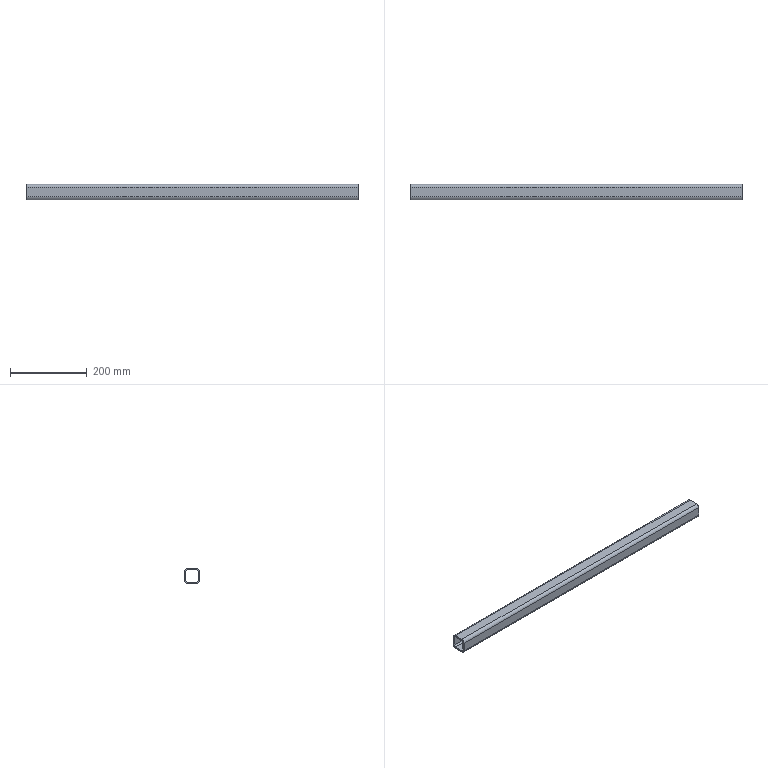Part | SolidWorks | features WeldMemberFeat 1, WeldmentFeature 1 | 1 solid | 18 faces | box 866 x 40 x 40 mm | volume 463134 mm3 | plane 10 | cylinder 8 | commonest cylinder face diameters 8 x4 16 x4
STEP:
#1=CARTESIAN_POINT('',(-433.,12.,-20.));
#2=VERTEX_POINT('',#1);
#3=CARTESIAN_POINT('',(-433.,20.,-12.));
#4=VERTEX_POINT('',#3);
#5=CARTESIAN_POINT('',(-433.,12.,-12.));
#6=DIRECTION('',(1.,0.,0.));
#7=DIRECTION('',(0.,0.,-1.));
#8=AXIS2_PLACEMENT_3D('',#5,#6,#7);
#9=CIRCLE('',#8,8.);
#10=EDGE_CURVE('',#2,#4,#9,.T.);
#11=ORIENTED_EDGE('',*,*,#10,.T.);
#12=CARTESIAN_POINT('',(433.,20.,-12.));
#13=VERTEX_POINT('',#12);
#14=CARTESIAN_POINT('',(433.,20.,-12.));
#15=DIRECTION('',(-1.,0.,0.));
#16=VECTOR('',#15,1000.);
#17=LINE('',#14,#16);
#18=EDGE_CURVE('',#13,#4,#17,.T.);
#19=ORIENTED_EDGE('',*,*,#18,.F.);
#20=CARTESIAN_POINT('',(433.,12.,-20.));
#21=VERTEX_POINT('',#20);
#22=CARTESIAN_POINT('',(433.,12.,-12.));
#23=DIRECTION('',(1.,0.,0.));
#24=DIRECTION('',(0.,0.,-1.));
#25=AXIS2_PLACEMENT_3D('',#22,#23,#24);
#26=CIRCLE('',#25,8.);
#27=EDGE_CURVE('',#21,#13,#26,.T.);
#28=ORIENTED_EDGE('',*,*,#27,.F.);
#29=CARTESIAN_POINT('',(433.,12.,-20.));
#30=DIRECTION('',(-1.,0.,0.));
#31=VECTOR('',#30,1000.);
#32=LINE('',#29,#31);
#33=EDGE_CURVE('',#21,#2,#32,.T.);
#34=ORIENTED_EDGE('',*,*,#33,.T.);
#35=EDGE_LOOP('',(#11,#19,#28,#34));
#36=FACE_OUTER_BOUND('',#35,.T.);
#37=CARTESIAN_POINT('',(433.,12.,-12.));
#38=DIRECTION('',(-1.,0.,0.));
#39=DIRECTION('',(0.,0.,1.));
#40=AXIS2_PLACEMENT_3D('',#37,#38,#39);
#41=CYLINDRICAL_SURFACE('',#40,8.);
#42=ADVANCED_FACE('',(#36),#41,.T.);
#43=CARTESIAN_POINT('',(-433.,20.,12.));
#44=VERTEX_POINT('',#43);
#45=CARTESIAN_POINT('',(-433.,20.,-12.));
#46=DIRECTION('',(0.,0.,1.));
#47=VECTOR('',#46,1000.);
#48=LINE('',#45,#47);
#49=EDGE_CURVE('',#4,#44,#48,.T.);
#50=ORIENTED_EDGE('',*,*,#49,.T.);
#51=CARTESIAN_POINT('',(433.,20.,12.));
#52=VERTEX_POINT('',#51);
#53=CARTESIAN_POINT('',(433.,20.,12.));
#54=DIRECTION('',(-1.,0.,0.));
#55=VECTOR('',#54,1000.);
#56=LINE('',#53,#55);
#57=EDGE_CURVE('',#52,#44,#56,.T.);
#58=ORIENTED_EDGE('',*,*,#57,.F.);
#59=CARTESIAN_POINT('',(433.,20.,-12.));
#60=DIRECTION('',(0.,0.,1.));
#61=VECTOR('',#60,1000.);
#62=LINE('',#59,#61);
#63=EDGE_CURVE('',#13,#52,#62,.T.);
#64=ORIENTED_EDGE('',*,*,#63,.F.);
#65=ORIENTED_EDGE('',*,*,#18,.T.);
#66=EDGE_LOOP('',(#50,#58,#64,#65));
#67=FACE_OUTER_BOUND('',#66,.T.);
#68=CARTESIAN_POINT('',(433.,20.,-12.));
#69=DIRECTION('',(0.,-1.,0.));
#70=DIRECTION('',(0.,0.,-1.));
#71=AXIS2_PLACEMENT_3D('',#68,#69,#70);
#72=PLANE('',#71);
#73=ADVANCED_FACE('',(#67),#72,.F.);
#74=CARTESIAN_POINT('',(-433.,12.,20.));
#75=VERTEX_POINT('',#74);
#76=CARTESIAN_POINT('',(-433.,12.,12.));
#77=DIRECTION('',(1.,0.,0.));
#78=DIRECTION('',(0.,0.,-1.));
#79=AXIS2_PLACEMENT_3D('',#76,#77,#78);
#80=CIRCLE('',#79,8.);
#81=EDGE_CURVE('',#44,#75,#80,.T.);
#82=ORIENTED_EDGE('',*,*,#81,.T.);
#83=CARTESIAN_POINT('',(433.,12.,20.));
#84=VERTEX_POINT('',#83);
#85=CARTESIAN_POINT('',(433.,12.,20.));
#86=DIRECTION('',(-1.,0.,0.));
#87=VECTOR('',#86,1000.);
#88=LINE('',#85,#87);
#89=EDGE_CURVE('',#84,#75,#88,.T.);
#90=ORIENTED_EDGE('',*,*,#89,.F.);
#91=CARTESIAN_POINT('',(433.,12.,12.));
#92=DIRECTION('',(1.,0.,0.));
#93=DIRECTION('',(0.,0.,-1.));
#94=AXIS2_PLACEMENT_3D('',#91,#92,#93);
#95=CIRCLE('',#94,8.);
#96=EDGE_CURVE('',#52,#84,#95,.T.);
#97=ORIENTED_EDGE('',*,*,#96,.F.);
#98=ORIENTED_EDGE('',*,*,#57,.T.);
#99=EDGE_LOOP('',(#82,#90,#97,#98));
#100=FACE_OUTER_BOUND('',#99,.T.);
#101=CARTESIAN_POINT('',(433.,12.,12.));
#102=DIRECTION('',(-1.,0.,0.));
#103=DIRECTION('',(0.,0.,1.));
#104=AXIS2_PLACEMENT_3D('',#101,#102,#103);
#105=CYLINDRICAL_SURFACE('',#104,8.);
#106=ADVANCED_FACE('',(#100),#105,.T.);
#107=CARTESIAN_POINT('',(-433.,-12.,20.));
#108=VERTEX_POINT('',#107);
#109=CARTESIAN_POINT('',(-433.,-12.,20.));
#110=DIRECTION('',(0.,-1.,0.));
#111=VECTOR('',#110,1000.);
#112=LINE('',#109,#111);
#113=EDGE_CURVE('',#75,#108,#112,.T.);
#114=ORIENTED_EDGE('',*,*,#113,.T.);
#115=CARTESIAN_POINT('',(433.,-12.,20.));
#116=VERTEX_POINT('',#115);
#117=CARTESIAN_POINT('',(433.,-12.,20.));
#118=DIRECTION('',(-1.,0.,0.));
#119=VECTOR('',#118,1000.);
#120=LINE('',#117,#119);
#121=EDGE_CURVE('',#116,#108,#120,.T.);
#122=ORIENTED_EDGE('',*,*,#121,.F.);
#123=CARTESIAN_POINT('',(433.,-12.,20.));
#124=DIRECTION('',(0.,-1.,0.));
#125=VECTOR('',#124,1000.);
#126=LINE('',#123,#125);
#127=EDGE_CURVE('',#84,#116,#126,.T.);
#128=ORIENTED_EDGE('',*,*,#127,.F.);
#129=ORIENTED_EDGE('',*,*,#89,.T.);
#130=EDGE_LOOP('',(#114,#122,#128,#129));
#131=FACE_OUTER_BOUND('',#130,.T.);
#132=CARTESIAN_POINT('',(433.,-12.,20.));
#133=DIRECTION('',(0.,0.,-1.));
#134=DIRECTION('',(-1.,0.,0.));
#135=AXIS2_PLACEMENT_3D('',#132,#133,#134);
#136=PLANE('',#135);
#137=ADVANCED_FACE('',(#131),#136,.F.);
#138=CARTESIAN_POINT('',(-433.,-20.,12.));
#139=VERTEX_POINT('',#138);
#140=CARTESIAN_POINT('',(-433.,-12.,12.));
#141=DIRECTION('',(1.,0.,0.));
#142=DIRECTION('',(0.,0.,-1.));
#143=AXIS2_PLACEMENT_3D('',#140,#141,#142);
#144=CIRCLE('',#143,8.);
#145=EDGE_CURVE('',#108,#139,#144,.T.);
#146=ORIENTED_EDGE('',*,*,#145,.T.);
#147=CARTESIAN_POINT('',(433.,-20.,12.));
#148=VERTEX_POINT('',#147);
#149=CARTESIAN_POINT('',(433.,-20.,12.));
#150=DIRECTION('',(-1.,0.,0.));
#151=VECTOR('',#150,1000.);
#152=LINE('',#149,#151);
#153=EDGE_CURVE('',#148,#139,#152,.T.);
#154=ORIENTED_EDGE('',*,*,#153,.F.);
#155=CARTESIAN_POINT('',(433.,-12.,12.));
#156=DIRECTION('',(1.,0.,0.));
#157=DIRECTION('',(0.,0.,-1.));
#158=AXIS2_PLACEMENT_3D('',#155,#156,#157);
#159=CIRCLE('',#158,8.);
#160=EDGE_CURVE('',#116,#148,#159,.T.);
#161=ORIENTED_EDGE('',*,*,#160,.F.);
#162=ORIENTED_EDGE('',*,*,#121,.T.);
#163=EDGE_LOOP('',(#146,#154,#161,#162));
#164=FACE_OUTER_BOUND('',#163,.T.);
#165=CARTESIAN_POINT('',(433.,-12.,12.));
#166=DIRECTION('',(-1.,0.,0.));
#167=DIRECTION('',(0.,0.,1.));
#168=AXIS2_PLACEMENT_3D('',#165,#166,#167);
#169=CYLINDRICAL_SURFACE('',#168,8.);
#170=ADVANCED_FACE('',(#164),#169,.T.);
#171=CARTESIAN_POINT('',(-433.,-20.,-12.));
#172=VERTEX_POINT('',#171);
#173=CARTESIAN_POINT('',(-433.,-20.,12.));
#174=DIRECTION('',(0.,0.,-1.));
#175=VECTOR('',#174,1000.);
#176=LINE('',#173,#175);
#177=EDGE_CURVE('',#139,#172,#176,.T.);
#178=ORIENTED_EDGE('',*,*,#177,.T.);
#179=CARTESIAN_POINT('',(433.,-20.,-12.));
#180=VERTEX_POINT('',#179);
#181=CARTESIAN_POINT('',(433.,-20.,-12.));
#182=DIRECTION('',(-1.,0.,0.));
#183=VECTOR('',#182,1000.);
#184=LINE('',#181,#183);
#185=EDGE_CURVE('',#180,#172,#184,.T.);
#186=ORIENTED_EDGE('',*,*,#185,.F.);
#187=CARTESIAN_POINT('',(433.,-20.,12.));
#188=DIRECTION('',(0.,0.,-1.));
#189=VECTOR('',#188,1000.);
#190=LINE('',#187,#189);
#191=EDGE_CURVE('',#148,#180,#190,.T.);
#192=ORIENTED_EDGE('',*,*,#191,.F.);
#193=ORIENTED_EDGE('',*,*,#153,.T.);
#194=EDGE_LOOP('',(#178,#186,#192,#193));
#195=FACE_OUTER_BOUND('',#194,.T.);
#196=CARTESIAN_POINT('',(433.,-20.,12.));
#197=DIRECTION('',(0.,1.,0.));
#198=DIRECTION('',(0.,0.,1.));
#199=AXIS2_PLACEMENT_3D('',#196,#197,#198);
#200=PLANE('',#199);
#201=ADVANCED_FACE('',(#195),#200,.F.);
#202=CARTESIAN_POINT('',(-433.,-12.,-20.));
#203=VERTEX_POINT('',#202);
#204=CARTESIAN_POINT('',(-433.,-12.,-12.));
#205=DIRECTION('',(1.,0.,0.));
#206=DIRECTION('',(0.,0.,-1.));
#207=AXIS2_PLACEMENT_3D('',#204,#205,#206);
#208=CIRCLE('',#207,8.);
#209=EDGE_CURVE('',#172,#203,#208,.T.);
#210=ORIENTED_EDGE('',*,*,#209,.T.);
#211=CARTESIAN_POINT('',(433.,-12.,-20.));
#212=VERTEX_POINT('',#211);
#213=CARTESIAN_POINT('',(433.,-12.,-20.));
#214=DIRECTION('',(-1.,0.,0.));
#215=VECTOR('',#214,1000.);
#216=LINE('',#213,#215);
#217=EDGE_CURVE('',#212,#203,#216,.T.);
#218=ORIENTED_EDGE('',*,*,#217,.F.);
#219=CARTESIAN_POINT('',(433.,-12.,-12.));
#220=DIRECTION('',(1.,0.,0.));
#221=DIRECTION('',(0.,0.,-1.));
#222=AXIS2_PLACEMENT_3D('',#219,#220,#221);
#223=CIRCLE('',#222,8.);
#224=EDGE_CURVE('',#180,#212,#223,.T.);
#225=ORIENTED_EDGE('',*,*,#224,.F.);
#226=ORIENTED_EDGE('',*,*,#185,.T.);
#227=EDGE_LOOP('',(#210,#218,#225,#226));
#228=FACE_OUTER_BOUND('',#227,.T.);
#229=CARTESIAN_POINT('',(433.,-12.,-12.));
#230=DIRECTION('',(-1.,0.,0.));
#231=DIRECTION('',(0.,0.,1.));
#232=AXIS2_PLACEMENT_3D('',#229,#230,#231);
#233=CYLINDRICAL_SURFACE('',#232,8.);
#234=ADVANCED_FACE('',(#228),#233,.T.);
#235=CARTESIAN_POINT('',(-433.,16.,12.));
#236=VERTEX_POINT('',#235);
#237=CARTESIAN_POINT('',(-433.,12.,16.));
#238=VERTEX_POINT('',#237);
#239=CARTESIAN_POINT('',(-433.,12.,12.));
#240=DIRECTION('',(1.,0.,0.));
#241=DIRECTION('',(0.,0.,-1.));
#242=AXIS2_PLACEMENT_3D('',#239,#240,#241);
#243=CIRCLE('',#242,4.);
#244=EDGE_CURVE('',#236,#238,#243,.T.);
#245=ORIENTED_EDGE('',*,*,#244,.F.);
#246=CARTESIAN_POINT('',(433.,16.,12.));
#247=VERTEX_POINT('',#246);
#248=CARTESIAN_POINT('',(433.,16.,12.));
#249=DIRECTION('',(-1.,0.,0.));
#250=VECTOR('',#249,1000.);
#251=LINE('',#248,#250);
#252=EDGE_CURVE('',#247,#236,#251,.T.);
#253=ORIENTED_EDGE('',*,*,#252,.F.);
#254=CARTESIAN_POINT('',(433.,12.,16.));
#255=VERTEX_POINT('',#254);
#256=CARTESIAN_POINT('',(433.,12.,12.));
#257=DIRECTION('',(1.,0.,0.));
#258=DIRECTION('',(0.,0.,-1.));
#259=AXIS2_PLACEMENT_3D('',#256,#257,#258);
#260=CIRCLE('',#259,4.);
#261=EDGE_CURVE('',#247,#255,#260,.T.);
#262=ORIENTED_EDGE('',*,*,#261,.T.);
#263=CARTESIAN_POINT('',(433.,12.,16.));
#264=DIRECTION('',(-1.,0.,0.));
#265=VECTOR('',#264,1000.);
#266=LINE('',#263,#265);
#267=EDGE_CURVE('',#255,#238,#266,.T.);
#268=ORIENTED_EDGE('',*,*,#267,.T.);
#269=EDGE_LOOP('',(#245,#253,#262,#268));
#270=FACE_OUTER_BOUND('',#269,.T.);
#271=CARTESIAN_POINT('',(433.,12.,12.));
#272=DIRECTION('',(-1.,0.,0.));
#273=DIRECTION('',(0.,0.,1.));
#274=AXIS2_PLACEMENT_3D('',#271,#272,#273);
#275=CYLINDRICAL_SURFACE('',#274,4.);
#276=ADVANCED_FACE('',(#270),#275,.F.);
#277=CARTESIAN_POINT('',(-433.,16.,-12.));
#278=VERTEX_POINT('',#277);
#279=CARTESIAN_POINT('',(-433.,16.,-12.));
#280=DIRECTION('',(0.,0.,1.));
#281=VECTOR('',#280,1000.);
#282=LINE('',#279,#281);
#283=EDGE_CURVE('',#278,#236,#282,.T.);
#284=ORIENTED_EDGE('',*,*,#283,.F.);
#285=CARTESIAN_POINT('',(433.,16.,-12.));
#286=VERTEX_POINT('',#285);
#287=CARTESIAN_POINT('',(433.,16.,-12.));
#288=DIRECTION('',(-1.,0.,0.));
#289=VECTOR('',#288,1000.);
#290=LINE('',#287,#289);
#291=EDGE_CURVE('',#286,#278,#290,.T.);
#292=ORIENTED_EDGE('',*,*,#291,.F.);
#293=CARTESIAN_POINT('',(433.,16.,-12.));
#294=DIRECTION('',(0.,0.,1.));
#295=VECTOR('',#294,1000.);
#296=LINE('',#293,#295);
#297=EDGE_CURVE('',#286,#247,#296,.T.);
#298=ORIENTED_EDGE('',*,*,#297,.T.);
#299=ORIENTED_EDGE('',*,*,#252,.T.);
#300=EDGE_LOOP('',(#284,#292,#298,#299));
#301=FACE_OUTER_BOUND('',#300,.T.);
#302=CARTESIAN_POINT('',(433.,16.,-12.));
#303=DIRECTION('',(0.,-1.,0.));
#304=DIRECTION('',(0.,0.,-1.));
#305=AXIS2_PLACEMENT_3D('',#302,#303,#304);
#306=PLANE('',#305);
#307=ADVANCED_FACE('',(#301),#306,.T.);
#308=CARTESIAN_POINT('',(-433.,12.,-16.));
#309=VERTEX_POINT('',#308);
#310=CARTESIAN_POINT('',(-433.,12.,-12.));
#311=DIRECTION('',(1.,0.,0.));
#312=DIRECTION('',(0.,0.,-1.));
#313=AXIS2_PLACEMENT_3D('',#310,#311,#312);
#314=CIRCLE('',#313,4.);
#315=EDGE_CURVE('',#309,#278,#314,.T.);
#316=ORIENTED_EDGE('',*,*,#315,.F.);
#317=CARTESIAN_POINT('',(433.,12.,-16.));
#318=VERTEX_POINT('',#317);
#319=CARTESIAN_POINT('',(433.,12.,-16.));
#320=DIRECTION('',(-1.,0.,0.));
#321=VECTOR('',#320,1000.);
#322=LINE('',#319,#321);
#323=EDGE_CURVE('',#318,#309,#322,.T.);
#324=ORIENTED_EDGE('',*,*,#323,.F.);
#325=CARTESIAN_POINT('',(433.,12.,-12.));
#326=DIRECTION('',(1.,0.,0.));
#327=DIRECTION('',(0.,0.,-1.));
#328=AXIS2_PLACEMENT_3D('',#325,#326,#327);
#329=CIRCLE('',#328,4.);
#330=EDGE_CURVE('',#318,#286,#329,.T.);
#331=ORIENTED_EDGE('',*,*,#330,.T.);
#332=ORIENTED_EDGE('',*,*,#291,.T.);
#333=EDGE_LOOP('',(#316,#324,#331,#332));
#334=FACE_OUTER_BOUND('',#333,.T.);
#335=CARTESIAN_POINT('',(433.,12.,-12.));
#336=DIRECTION('',(-1.,0.,0.));
#337=DIRECTION('',(0.,0.,1.));
#338=AXIS2_PLACEMENT_3D('',#335,#336,#337);
#339=CYLINDRICAL_SURFACE('',#338,4.);
#340=ADVANCED_FACE('',(#334),#339,.F.);
#341=CARTESIAN_POINT('',(-433.,-12.,-16.));
#342=VERTEX_POINT('',#341);
#343=CARTESIAN_POINT('',(-433.,12.,-16.));
#344=DIRECTION('',(0.,1.,0.));
#345=VECTOR('',#344,1000.);
#346=LINE('',#343,#345);
#347=EDGE_CURVE('',#342,#309,#346,.T.);
#348=ORIENTED_EDGE('',*,*,#347,.F.);
#349=CARTESIAN_POINT('',(433.,-12.,-16.));
#350=VERTEX_POINT('',#349);
#351=CARTESIAN_POINT('',(433.,-12.,-16.));
#352=DIRECTION('',(-1.,0.,0.));
#353=VECTOR('',#352,1000.);
#354=LINE('',#351,#353);
#355=EDGE_CURVE('',#350,#342,#354,.T.);
#356=ORIENTED_EDGE('',*,*,#355,.F.);
#357=CARTESIAN_POINT('',(433.,12.,-16.));
#358=DIRECTION('',(0.,1.,0.));
#359=VECTOR('',#358,1000.);
#360=LINE('',#357,#359);
#361=EDGE_CURVE('',#350,#318,#360,.T.);
#362=ORIENTED_EDGE('',*,*,#361,.T.);
#363=ORIENTED_EDGE('',*,*,#323,.T.);
#364=EDGE_LOOP('',(#348,#356,#362,#363));
#365=FACE_OUTER_BOUND('',#364,.T.);
#366=CARTESIAN_POINT('',(433.,12.,-16.));
#367=DIRECTION('',(0.,0.,1.));
#368=DIRECTION('',(1.,0.,0.));
#369=AXIS2_PLACEMENT_3D('',#366,#367,#368);
#370=PLANE('',#369);
#371=ADVANCED_FACE('',(#365),#370,.T.);
#372=CARTESIAN_POINT('',(-433.,-16.,-12.));
#373=VERTEX_POINT('',#372);
#374=CARTESIAN_POINT('',(-433.,-12.,-12.));
#375=DIRECTION('',(1.,0.,0.));
#376=DIRECTION('',(0.,0.,-1.));
#377=AXIS2_PLACEMENT_3D('',#374,#375,#376);
#378=CIRCLE('',#377,4.);
#379=EDGE_CURVE('',#373,#342,#378,.T.);
#380=ORIENTED_EDGE('',*,*,#379,.F.);
#381=CARTESIAN_POINT('',(433.,-16.,-12.));
#382=VERTEX_POINT('',#381);
#383=CARTESIAN_POINT('',(433.,-16.,-12.));
#384=DIRECTION('',(-1.,0.,0.));
#385=VECTOR('',#384,1000.);
#386=LINE('',#383,#385);
#387=EDGE_CURVE('',#382,#373,#386,.T.);
#388=ORIENTED_EDGE('',*,*,#387,.F.);
#389=CARTESIAN_POINT('',(433.,-12.,-12.));
#390=DIRECTION('',(1.,0.,0.));
#391=DIRECTION('',(0.,0.,-1.));
#392=AXIS2_PLACEMENT_3D('',#389,#390,#391);
#393=CIRCLE('',#392,4.);
#394=EDGE_CURVE('',#382,#350,#393,.T.);
#395=ORIENTED_EDGE('',*,*,#394,.T.);
#396=ORIENTED_EDGE('',*,*,#355,.T.);
#397=EDGE_LOOP('',(#380,#388,#395,#396));
#398=FACE_OUTER_BOUND('',#397,.T.);
#399=CARTESIAN_POINT('',(433.,-12.,-12.));
#400=DIRECTION('',(-1.,0.,0.));
#401=DIRECTION('',(0.,0.,1.));
#402=AXIS2_PLACEMENT_3D('',#399,#400,#401);
#403=CYLINDRICAL_SURFACE('',#402,4.);
#404=ADVANCED_FACE('',(#398),#403,.F.);
#405=CARTESIAN_POINT('',(-433.,-16.,12.));
#406=VERTEX_POINT('',#405);
#407=CARTESIAN_POINT('',(-433.,-16.,12.));
#408=DIRECTION('',(0.,0.,-1.));
#409=VECTOR('',#408,1000.);
#410=LINE('',#407,#409);
#411=EDGE_CURVE('',#406,#373,#410,.T.);
#412=ORIENTED_EDGE('',*,*,#411,.F.);
#413=CARTESIAN_POINT('',(433.,-16.,12.));
#414=VERTEX_POINT('',#413);
#415=CARTESIAN_POINT('',(433.,-16.,12.));
#416=DIRECTION('',(-1.,0.,0.));
#417=VECTOR('',#416,1000.);
#418=LINE('',#415,#417);
#419=EDGE_CURVE('',#414,#406,#418,.T.);
#420=ORIENTED_EDGE('',*,*,#419,.F.);
#421=CARTESIAN_POINT('',(433.,-16.,12.));
#422=DIRECTION('',(0.,0.,-1.));
#423=VECTOR('',#422,1000.);
#424=LINE('',#421,#423);
#425=EDGE_CURVE('',#414,#382,#424,.T.);
#426=ORIENTED_EDGE('',*,*,#425,.T.);
#427=ORIENTED_EDGE('',*,*,#387,.T.);
#428=EDGE_LOOP('',(#412,#420,#426,#427));
#429=FACE_OUTER_BOUND('',#428,.T.);
#430=CARTESIAN_POINT('',(433.,-16.,12.));
#431=DIRECTION('',(0.,1.,0.));
#432=DIRECTION('',(0.,0.,1.));
#433=AXIS2_PLACEMENT_3D('',#430,#431,#432);
#434=PLANE('',#433);
#435=ADVANCED_FACE('',(#429),#434,.T.);
#436=CARTESIAN_POINT('',(-433.,-12.,16.));
#437=VERTEX_POINT('',#436);
#438=CARTESIAN_POINT('',(-433.,-12.,12.));
#439=DIRECTION('',(1.,0.,0.));
#440=DIRECTION('',(0.,0.,-1.));
#441=AXIS2_PLACEMENT_3D('',#438,#439,#440);
#442=CIRCLE('',#441,4.);
#443=EDGE_CURVE('',#437,#406,#442,.T.);
#444=ORIENTED_EDGE('',*,*,#443,.F.);
#445=CARTESIAN_POINT('',(433.,-12.,16.));
#446=VERTEX_POINT('',#445);
#447=CARTESIAN_POINT('',(433.,-12.,16.));
#448=DIRECTION('',(-1.,0.,0.));
#449=VECTOR('',#448,1000.);
#450=LINE('',#447,#449);
#451=EDGE_CURVE('',#446,#437,#450,.T.);
#452=ORIENTED_EDGE('',*,*,#451,.F.);
#453=CARTESIAN_POINT('',(433.,-12.,12.));
#454=DIRECTION('',(1.,0.,0.));
#455=DIRECTION('',(0.,0.,-1.));
#456=AXIS2_PLACEMENT_3D('',#453,#454,#455);
#457=CIRCLE('',#456,4.);
#458=EDGE_CURVE('',#446,#414,#457,.T.);
#459=ORIENTED_EDGE('',*,*,#458,.T.);
#460=ORIENTED_EDGE('',*,*,#419,.T.);
#461=EDGE_LOOP('',(#444,#452,#459,#460));
#462=FACE_OUTER_BOUND('',#461,.T.);
#463=CARTESIAN_POINT('',(433.,-12.,12.));
#464=DIRECTION('',(-1.,0.,0.));
#465=DIRECTION('',(0.,0.,1.));
#466=AXIS2_PLACEMENT_3D('',#463,#464,#465);
#467=CYLINDRICAL_SURFACE('',#466,4.);
#468=ADVANCED_FACE('',(#462),#467,.F.);
#469=CARTESIAN_POINT('',(-433.,-12.,16.));
#470=DIRECTION('',(0.,-1.,0.));
#471=VECTOR('',#470,1000.);
#472=LINE('',#469,#471);
#473=EDGE_CURVE('',#238,#437,#472,.T.);
#474=ORIENTED_EDGE('',*,*,#473,.F.);
#475=ORIENTED_EDGE('',*,*,#267,.F.);
#476=CARTESIAN_POINT('',(433.,-12.,16.));
#477=DIRECTION('',(0.,-1.,0.));
#478=VECTOR('',#477,1000.);
#479=LINE('',#476,#478);
#480=EDGE_CURVE('',#255,#446,#479,.T.);
#481=ORIENTED_EDGE('',*,*,#480,.T.);
#482=ORIENTED_EDGE('',*,*,#451,.T.);
#483=EDGE_LOOP('',(#474,#475,#481,#482));
#484=FACE_OUTER_BOUND('',#483,.T.);
#485=CARTESIAN_POINT('',(433.,-12.,16.));
#486=DIRECTION('',(0.,0.,-1.));
#487=DIRECTION('',(-1.,0.,0.));
#488=AXIS2_PLACEMENT_3D('',#485,#486,#487);
#489=PLANE('',#488);
#490=ADVANCED_FACE('',(#484),#489,.T.);
#491=CARTESIAN_POINT('',(-433.,12.,-20.));
#492=DIRECTION('',(0.,1.,0.));
#493=VECTOR('',#492,1000.);
#494=LINE('',#491,#493);
#495=EDGE_CURVE('',#203,#2,#494,.T.);
#496=ORIENTED_EDGE('',*,*,#495,.T.);
#497=ORIENTED_EDGE('',*,*,#33,.F.);
#498=CARTESIAN_POINT('',(433.,12.,-20.));
#499=DIRECTION('',(0.,1.,0.));
#500=VECTOR('',#499,1000.);
#501=LINE('',#498,#500);
#502=EDGE_CURVE('',#212,#21,#501,.T.);
#503=ORIENTED_EDGE('',*,*,#502,.F.);
#504=ORIENTED_EDGE('',*,*,#217,.T.);
#505=EDGE_LOOP('',(#496,#497,#503,#504));
#506=FACE_OUTER_BOUND('',#505,.T.);
#507=CARTESIAN_POINT('',(433.,12.,-20.));
#508=DIRECTION('',(0.,0.,1.));
#509=DIRECTION('',(1.,0.,0.));
#510=AXIS2_PLACEMENT_3D('',#507,#508,#509);
#511=PLANE('',#510);
#512=ADVANCED_FACE('',(#506),#511,.F.);
#513=ORIENTED_EDGE('',*,*,#261,.F.);
#514=ORIENTED_EDGE('',*,*,#297,.F.);
#515=ORIENTED_EDGE('',*,*,#330,.F.);
#516=ORIENTED_EDGE('',*,*,#361,.F.);
#517=ORIENTED_EDGE('',*,*,#394,.F.);
#518=ORIENTED_EDGE('',*,*,#425,.F.);
#519=ORIENTED_EDGE('',*,*,#458,.F.);
#520=ORIENTED_EDGE('',*,*,#480,.F.);
#521=EDGE_LOOP('',(#513,#514,#515,#516,#517,#518,#519,#520));
#522=FACE_BOUND('',#521,.T.);
#523=ORIENTED_EDGE('',*,*,#27,.T.);
#524=ORIENTED_EDGE('',*,*,#63,.T.);
#525=ORIENTED_EDGE('',*,*,#96,.T.);
#526=ORIENTED_EDGE('',*,*,#127,.T.);
#527=ORIENTED_EDGE('',*,*,#160,.T.);
#528=ORIENTED_EDGE('',*,*,#191,.T.);
#529=ORIENTED_EDGE('',*,*,#224,.T.);
#530=ORIENTED_EDGE('',*,*,#502,.T.);
#531=EDGE_LOOP('',(#523,#524,#525,#526,#527,#528,#529,#530));
#532=FACE_OUTER_BOUND('',#531,.T.);
#533=CARTESIAN_POINT('',(433.,12.,-12.));
#534=DIRECTION('',(1.,0.,0.));
#535=DIRECTION('',(0.,0.,-1.));
#536=AXIS2_PLACEMENT_3D('',#533,#534,#535);
#537=PLANE('',#536);
#538=ADVANCED_FACE('',(#522,#532),#537,.T.);
#539=ORIENTED_EDGE('',*,*,#244,.T.);
#540=ORIENTED_EDGE('',*,*,#473,.T.);
#541=ORIENTED_EDGE('',*,*,#443,.T.);
#542=ORIENTED_EDGE('',*,*,#411,.T.);
#543=ORIENTED_EDGE('',*,*,#379,.T.);
#544=ORIENTED_EDGE('',*,*,#347,.T.);
#545=ORIENTED_EDGE('',*,*,#315,.T.);
#546=ORIENTED_EDGE('',*,*,#283,.T.);
#547=EDGE_LOOP('',(#539,#540,#541,#542,#543,#544,#545,#546));
#548=FACE_BOUND('',#547,.T.);
#549=ORIENTED_EDGE('',*,*,#10,.F.);
#550=ORIENTED_EDGE('',*,*,#495,.F.);
#551=ORIENTED_EDGE('',*,*,#209,.F.);
#552=ORIENTED_EDGE('',*,*,#177,.F.);
#553=ORIENTED_EDGE('',*,*,#145,.F.);
#554=ORIENTED_EDGE('',*,*,#113,.F.);
#555=ORIENTED_EDGE('',*,*,#81,.F.);
#556=ORIENTED_EDGE('',*,*,#49,.F.);
#557=EDGE_LOOP('',(#549,#550,#551,#552,#553,#554,#555,#556));
#558=FACE_OUTER_BOUND('',#557,.T.);
#559=CARTESIAN_POINT('',(-433.,12.,-12.));
#560=DIRECTION('',(1.,0.,0.));
#561=DIRECTION('',(0.,0.,-1.));
#562=AXIS2_PLACEMENT_3D('',#559,#560,#561);
#563=PLANE('',#562);
#564=ADVANCED_FACE('',(#548,#558),#563,.F.);
#565=CLOSED_SHELL('',(#42,#73,#106,#137,#170,#201,#234,#276,#307,#340,#371,#404,#435,#468,#490,#512,#538,#564));
#566=MANIFOLD_SOLID_BREP('',#565);
#567=CARTESIAN_POINT('',(0.,0.,0.));
#568=DIRECTION('',(0.,0.,1.));
#569=DIRECTION('',(1.,0.,0.));
#570=AXIS2_PLACEMENT_3D('',#567,#568,#569);
#571=(LENGTH_UNIT()NAMED_UNIT(*)SI_UNIT(.MILLI.,.METRE.));
#572=UNCERTAINTY_MEASURE_WITH_UNIT(LENGTH_MEASURE(0.00001),#571,'','');
#573=(NAMED_UNIT(*)PLANE_ANGLE_UNIT()SI_UNIT($,.RADIAN.));
#574=(NAMED_UNIT(*)SI_UNIT($,.STERADIAN.)SOLID_ANGLE_UNIT());
#575=(GEOMETRIC_REPRESENTATION_CONTEXT(3)GLOBAL_UNCERTAINTY_ASSIGNED_CONTEXT((#572))GLOBAL_UNIT_ASSIGNED_CONTEXT((#571,#573,#574))REPRESENTATION_CONTEXT('',''));
#576=ADVANCED_BREP_SHAPE_REPRESENTATION('',(#566,#570),#575);